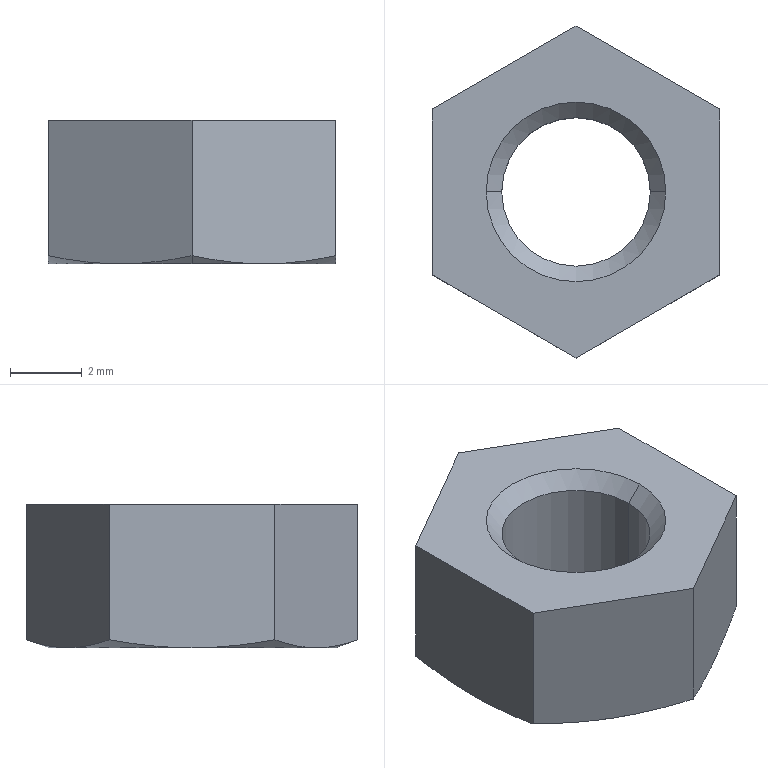Part | SolidWorks | features BaseBody 1 | 1 solid | 21 faces | box 8 x 9.238 x 4 mm | volume 165.049 mm3 | cone 11 | plane 8 | cylinder 2 | commonest cylinder face diameters 4.134 x2
STEP:
#1=CARTESIAN_POINT('',(-2.067,0.,0.433));
#2=VERTEX_POINT('',#1);
#3=CARTESIAN_POINT('',(2.067,0.,0.433));
#4=VERTEX_POINT('',#3);
#5=CARTESIAN_POINT('',(0.,0.,0.433));
#6=DIRECTION('',(0.,0.,1.));
#7=DIRECTION('',(1.,0.,0.));
#8=AXIS2_PLACEMENT_3D('',#5,#6,#7);
#9=CIRCLE('',#8,2.067);
#10=EDGE_CURVE('',#2,#4,#9,.T.);
#11=ORIENTED_EDGE('',*,*,#10,.F.);
#12=CARTESIAN_POINT('',(-2.067,0.,3.567));
#13=VERTEX_POINT('',#12);
#14=CARTESIAN_POINT('',(-2.067,0.,0.));
#15=DIRECTION('',(0.,0.,1.));
#16=VECTOR('',#15,1000.);
#17=LINE('',#14,#16);
#18=EDGE_CURVE('',#2,#13,#17,.T.);
#19=ORIENTED_EDGE('',*,*,#18,.T.);
#20=CARTESIAN_POINT('',(2.067,0.,3.567));
#21=VERTEX_POINT('',#20);
#22=CARTESIAN_POINT('',(0.,0.,3.567));
#23=DIRECTION('',(0.,0.,-1.));
#24=DIRECTION('',(1.,0.,0.));
#25=AXIS2_PLACEMENT_3D('',#22,#23,#24);
#26=CIRCLE('',#25,2.067);
#27=EDGE_CURVE('',#21,#13,#26,.T.);
#28=ORIENTED_EDGE('',*,*,#27,.F.);
#29=CARTESIAN_POINT('',(2.067,0.,0.));
#30=DIRECTION('',(0.,0.,1.));
#31=VECTOR('',#30,1000.);
#32=LINE('',#29,#31);
#33=EDGE_CURVE('',#4,#21,#32,.T.);
#34=ORIENTED_EDGE('',*,*,#33,.F.);
#35=EDGE_LOOP('',(#11,#19,#28,#34));
#36=FACE_OUTER_BOUND('',#35,.T.);
#37=CARTESIAN_POINT('',(0.,0.,0.));
#38=DIRECTION('',(0.,0.,1.));
#39=DIRECTION('',(1.,0.,0.));
#40=AXIS2_PLACEMENT_3D('',#37,#38,#39);
#41=CYLINDRICAL_SURFACE('',#40,2.067);
#42=ADVANCED_FACE('',(#36),#41,.F.);
#43=ORIENTED_EDGE('',*,*,#27,.T.);
#44=CARTESIAN_POINT('',(-2.5,0.,4.));
#45=VERTEX_POINT('',#44);
#46=CARTESIAN_POINT('',(-2.5,0.,4.));
#47=DIRECTION('',(-0.7071,0.,0.7071));
#48=VECTOR('',#47,1000.);
#49=LINE('',#46,#48);
#50=EDGE_CURVE('',#13,#45,#49,.T.);
#51=ORIENTED_EDGE('',*,*,#50,.T.);
#52=CARTESIAN_POINT('',(2.5,0.,4.));
#53=VERTEX_POINT('',#52);
#54=CARTESIAN_POINT('',(0.,0.,4.));
#55=DIRECTION('',(0.,0.,-1.));
#56=DIRECTION('',(1.,0.,0.));
#57=AXIS2_PLACEMENT_3D('',#54,#55,#56);
#58=CIRCLE('',#57,2.5);
#59=EDGE_CURVE('',#53,#45,#58,.T.);
#60=ORIENTED_EDGE('',*,*,#59,.F.);
#61=CARTESIAN_POINT('',(2.5,0.,4.));
#62=DIRECTION('',(0.7071,0.,0.7071));
#63=VECTOR('',#62,1000.);
#64=LINE('',#61,#63);
#65=EDGE_CURVE('',#21,#53,#64,.T.);
#66=ORIENTED_EDGE('',*,*,#65,.F.);
#67=EDGE_LOOP('',(#43,#51,#60,#66));
#68=FACE_OUTER_BOUND('',#67,.T.);
#69=CARTESIAN_POINT('',(0.,0.,4.));
#70=DIRECTION('',(0.,0.,1.));
#71=DIRECTION('',(1.,0.,0.));
#72=AXIS2_PLACEMENT_3D('',#69,#70,#71);
#73=CONICAL_SURFACE('',#72,2.5,0.7854);
#74=ADVANCED_FACE('',(#68),#73,.F.);
#75=ORIENTED_EDGE('',*,*,#10,.T.);
#76=CARTESIAN_POINT('',(2.5,0.,0.));
#77=VERTEX_POINT('',#76);
#78=CARTESIAN_POINT('',(2.5,0.,0.));
#79=DIRECTION('',(0.7071,0.,-0.7071));
#80=VECTOR('',#79,1000.);
#81=LINE('',#78,#80);
#82=EDGE_CURVE('',#4,#77,#81,.T.);
#83=ORIENTED_EDGE('',*,*,#82,.T.);
#84=CARTESIAN_POINT('',(-2.5,0.,0.));
#85=VERTEX_POINT('',#84);
#86=CARTESIAN_POINT('',(0.,0.,0.));
#87=DIRECTION('',(0.,0.,1.));
#88=DIRECTION('',(-1.,0.,0.));
#89=AXIS2_PLACEMENT_3D('',#86,#87,#88);
#90=CIRCLE('',#89,2.5);
#91=EDGE_CURVE('',#85,#77,#90,.T.);
#92=ORIENTED_EDGE('',*,*,#91,.F.);
#93=CARTESIAN_POINT('',(-2.5,0.,0.));
#94=DIRECTION('',(-0.7071,0.,-0.7071));
#95=VECTOR('',#94,1000.);
#96=LINE('',#93,#95);
#97=EDGE_CURVE('',#2,#85,#96,.T.);
#98=ORIENTED_EDGE('',*,*,#97,.F.);
#99=EDGE_LOOP('',(#75,#83,#92,#98));
#100=FACE_OUTER_BOUND('',#99,.T.);
#101=CARTESIAN_POINT('',(0.,0.,0.));
#102=DIRECTION('',(0.,0.,-1.));
#103=DIRECTION('',(-1.,0.,0.));
#104=AXIS2_PLACEMENT_3D('',#101,#102,#103);
#105=CONICAL_SURFACE('',#104,2.5,0.7854);
#106=ADVANCED_FACE('',(#100),#105,.F.);
#107=CARTESIAN_POINT('',(-2.,-3.464,0.));
#108=VERTEX_POINT('',#107);
#109=CARTESIAN_POINT('',(0.,-4.,0.));
#110=VERTEX_POINT('',#109);
#111=CARTESIAN_POINT('',(0.,0.,0.));
#112=DIRECTION('',(0.,0.,1.));
#113=DIRECTION('',(0.,-1.,0.));
#114=AXIS2_PLACEMENT_3D('',#111,#112,#113);
#115=CIRCLE('',#114,4.);
#116=EDGE_CURVE('',#108,#110,#115,.T.);
#117=ORIENTED_EDGE('',*,*,#116,.T.);
#118=CARTESIAN_POINT('',(0.,-4.619,0.2252));
#119=VERTEX_POINT('',#118);
#120=CARTESIAN_POINT('',(0.,-4.623,0.2266));
#121=DIRECTION('',(0.,-0.9397,0.342));
#122=VECTOR('',#121,1000.);
#123=LINE('',#120,#122);
#124=EDGE_CURVE('',#110,#119,#123,.T.);
#125=ORIENTED_EDGE('',*,*,#124,.T.);
#126=CARTESIAN_POINT('',(0.,-4.619,0.2252));
#127=CARTESIAN_POINT('',(-0.6613,-4.237,0.08627));
#128=CARTESIAN_POINT('',(-1.327,-3.853,0.));
#129=CARTESIAN_POINT('',(-2.,-3.464,0.));
#130=B_SPLINE_CURVE_WITH_KNOTS('',3,(#126,#127,#128,#129),.UNSPECIFIED.,.F.,.F.,(4,4),(0.,0.00232),.UNSPECIFIED.);
#131=EDGE_CURVE('',#119,#108,#130,.T.);
#132=ORIENTED_EDGE('',*,*,#131,.T.);
#133=EDGE_LOOP('',(#117,#125,#132));
#134=FACE_OUTER_BOUND('',#133,.T.);
#135=CARTESIAN_POINT('',(0.,0.,0.2266));
#136=DIRECTION('',(0.,0.,1.));
#137=DIRECTION('',(0.,-1.,0.));
#138=AXIS2_PLACEMENT_3D('',#135,#136,#137);
#139=CONICAL_SURFACE('',#138,4.623,1.222);
#140=ADVANCED_FACE('',(#134),#139,.T.);
#141=ORIENTED_EDGE('',*,*,#18,.F.);
#142=CARTESIAN_POINT('',(0.,0.,0.433));
#143=DIRECTION('',(0.,0.,1.));
#144=DIRECTION('',(1.,0.,0.));
#145=AXIS2_PLACEMENT_3D('',#142,#143,#144);
#146=CIRCLE('',#145,2.067);
#147=EDGE_CURVE('',#4,#2,#146,.T.);
#148=ORIENTED_EDGE('',*,*,#147,.F.);
#149=ORIENTED_EDGE('',*,*,#33,.T.);
#150=CARTESIAN_POINT('',(0.,0.,3.567));
#151=DIRECTION('',(0.,0.,-1.));
#152=DIRECTION('',(1.,0.,0.));
#153=AXIS2_PLACEMENT_3D('',#150,#151,#152);
#154=CIRCLE('',#153,2.067);
#155=EDGE_CURVE('',#13,#21,#154,.T.);
#156=ORIENTED_EDGE('',*,*,#155,.F.);
#157=EDGE_LOOP('',(#141,#148,#149,#156));
#158=FACE_OUTER_BOUND('',#157,.T.);
#159=CARTESIAN_POINT('',(0.,0.,0.));
#160=DIRECTION('',(0.,0.,1.));
#161=DIRECTION('',(1.,0.,0.));
#162=AXIS2_PLACEMENT_3D('',#159,#160,#161);
#163=CYLINDRICAL_SURFACE('',#162,2.067);
#164=ADVANCED_FACE('',(#158),#163,.F.);
#165=ORIENTED_EDGE('',*,*,#50,.F.);
#166=ORIENTED_EDGE('',*,*,#155,.T.);
#167=ORIENTED_EDGE('',*,*,#65,.T.);
#168=CARTESIAN_POINT('',(0.,0.,4.));
#169=DIRECTION('',(0.,0.,-1.));
#170=DIRECTION('',(1.,0.,0.));
#171=AXIS2_PLACEMENT_3D('',#168,#169,#170);
#172=CIRCLE('',#171,2.5);
#173=EDGE_CURVE('',#45,#53,#172,.T.);
#174=ORIENTED_EDGE('',*,*,#173,.F.);
#175=EDGE_LOOP('',(#165,#166,#167,#174));
#176=FACE_OUTER_BOUND('',#175,.T.);
#177=CARTESIAN_POINT('',(0.,0.,4.));
#178=DIRECTION('',(0.,0.,1.));
#179=DIRECTION('',(1.,0.,0.));
#180=AXIS2_PLACEMENT_3D('',#177,#178,#179);
#181=CONICAL_SURFACE('',#180,2.5,0.7854);
#182=ADVANCED_FACE('',(#176),#181,.F.);
#183=ORIENTED_EDGE('',*,*,#82,.F.);
#184=ORIENTED_EDGE('',*,*,#147,.T.);
#185=ORIENTED_EDGE('',*,*,#97,.T.);
#186=CARTESIAN_POINT('',(0.,0.,0.));
#187=DIRECTION('',(0.,0.,1.));
#188=DIRECTION('',(-1.,0.,0.));
#189=AXIS2_PLACEMENT_3D('',#186,#187,#188);
#190=CIRCLE('',#189,2.5);
#191=EDGE_CURVE('',#77,#85,#190,.T.);
#192=ORIENTED_EDGE('',*,*,#191,.F.);
#193=EDGE_LOOP('',(#183,#184,#185,#192));
#194=FACE_OUTER_BOUND('',#193,.T.);
#195=CARTESIAN_POINT('',(0.,0.,0.));
#196=DIRECTION('',(0.,0.,-1.));
#197=DIRECTION('',(-1.,0.,0.));
#198=AXIS2_PLACEMENT_3D('',#195,#196,#197);
#199=CONICAL_SURFACE('',#198,2.5,0.7854);
#200=ADVANCED_FACE('',(#194),#199,.F.);
#201=ORIENTED_EDGE('',*,*,#59,.T.);
#202=ORIENTED_EDGE('',*,*,#173,.T.);
#203=EDGE_LOOP('',(#201,#202));
#204=FACE_BOUND('',#203,.T.);
#205=CARTESIAN_POINT('',(4.,-2.309,4.));
#206=VERTEX_POINT('',#205);
#207=CARTESIAN_POINT('',(4.,2.309,4.));
#208=VERTEX_POINT('',#207);
#209=CARTESIAN_POINT('',(4.,0.,4.));
#210=DIRECTION('',(0.,1.,0.));
#211=VECTOR('',#210,1000.);
#212=LINE('',#209,#211);
#213=EDGE_CURVE('',#206,#208,#212,.T.);
#214=ORIENTED_EDGE('',*,*,#213,.T.);
#215=CARTESIAN_POINT('',(0.,4.619,4.));
#216=VERTEX_POINT('',#215);
#217=CARTESIAN_POINT('',(4.,2.309,4.));
#218=DIRECTION('',(-0.866,0.5,0.));
#219=VECTOR('',#218,1000.);
#220=LINE('',#217,#219);
#221=EDGE_CURVE('',#208,#216,#220,.T.);
#222=ORIENTED_EDGE('',*,*,#221,.T.);
#223=CARTESIAN_POINT('',(-4.,2.309,4.));
#224=VERTEX_POINT('',#223);
#225=CARTESIAN_POINT('',(0.,4.619,4.));
#226=DIRECTION('',(-0.866,-0.5,0.));
#227=VECTOR('',#226,1000.);
#228=LINE('',#225,#227);
#229=EDGE_CURVE('',#216,#224,#228,.T.);
#230=ORIENTED_EDGE('',*,*,#229,.T.);
#231=CARTESIAN_POINT('',(-4.,-2.309,4.));
#232=VERTEX_POINT('',#231);
#233=CARTESIAN_POINT('',(-4.,0.,4.));
#234=DIRECTION('',(0.,-1.,0.));
#235=VECTOR('',#234,1000.);
#236=LINE('',#233,#235);
#237=EDGE_CURVE('',#224,#232,#236,.T.);
#238=ORIENTED_EDGE('',*,*,#237,.T.);
#239=CARTESIAN_POINT('',(0.,-4.619,4.));
#240=VERTEX_POINT('',#239);
#241=CARTESIAN_POINT('',(-4.,-2.309,4.));
#242=DIRECTION('',(0.866,-0.5,0.));
#243=VECTOR('',#242,1000.);
#244=LINE('',#241,#243);
#245=EDGE_CURVE('',#232,#240,#244,.T.);
#246=ORIENTED_EDGE('',*,*,#245,.T.);
#247=CARTESIAN_POINT('',(0.,-4.619,4.));
#248=DIRECTION('',(0.866,0.5,0.));
#249=VECTOR('',#248,1000.);
#250=LINE('',#247,#249);
#251=EDGE_CURVE('',#240,#206,#250,.T.);
#252=ORIENTED_EDGE('',*,*,#251,.T.);
#253=EDGE_LOOP('',(#214,#222,#230,#238,#246,#252));
#254=FACE_OUTER_BOUND('',#253,.T.);
#255=CARTESIAN_POINT('',(0.,0.,4.));
#256=DIRECTION('',(0.,0.,1.));
#257=DIRECTION('',(1.,0.,0.));
#258=AXIS2_PLACEMENT_3D('',#255,#256,#257);
#259=PLANE('',#258);
#260=ADVANCED_FACE('',(#204,#254),#259,.T.);
#261=ORIENTED_EDGE('',*,*,#91,.T.);
#262=ORIENTED_EDGE('',*,*,#191,.T.);
#263=EDGE_LOOP('',(#261,#262));
#264=FACE_BOUND('',#263,.T.);
#265=ORIENTED_EDGE('',*,*,#116,.F.);
#266=CARTESIAN_POINT('',(-4.,0.,0.));
#267=VERTEX_POINT('',#266);
#268=CARTESIAN_POINT('',(0.,0.,0.));
#269=DIRECTION('',(0.,0.,1.));
#270=DIRECTION('',(0.,-1.,0.));
#271=AXIS2_PLACEMENT_3D('',#268,#269,#270);
#272=CIRCLE('',#271,4.);
#273=EDGE_CURVE('',#267,#108,#272,.T.);
#274=ORIENTED_EDGE('',*,*,#273,.F.);
#275=CARTESIAN_POINT('',(-2.,3.464,0.));
#276=VERTEX_POINT('',#275);
#277=CARTESIAN_POINT('',(0.,0.,0.));
#278=DIRECTION('',(0.,0.,1.));
#279=DIRECTION('',(0.,-1.,0.));
#280=AXIS2_PLACEMENT_3D('',#277,#278,#279);
#281=CIRCLE('',#280,4.);
#282=EDGE_CURVE('',#276,#267,#281,.T.);
#283=ORIENTED_EDGE('',*,*,#282,.F.);
#284=CARTESIAN_POINT('',(2.,3.464,0.));
#285=VERTEX_POINT('',#284);
#286=CARTESIAN_POINT('',(0.,0.,0.));
#287=DIRECTION('',(0.,0.,1.));
#288=DIRECTION('',(0.,-1.,0.));
#289=AXIS2_PLACEMENT_3D('',#286,#287,#288);
#290=CIRCLE('',#289,4.);
#291=EDGE_CURVE('',#285,#276,#290,.T.);
#292=ORIENTED_EDGE('',*,*,#291,.F.);
#293=CARTESIAN_POINT('',(4.,0.,0.));
#294=VERTEX_POINT('',#293);
#295=CARTESIAN_POINT('',(0.,0.,0.));
#296=DIRECTION('',(0.,0.,1.));
#297=DIRECTION('',(0.,-1.,0.));
#298=AXIS2_PLACEMENT_3D('',#295,#296,#297);
#299=CIRCLE('',#298,4.);
#300=EDGE_CURVE('',#294,#285,#299,.T.);
#301=ORIENTED_EDGE('',*,*,#300,.F.);
#302=CARTESIAN_POINT('',(2.,-3.464,0.));
#303=VERTEX_POINT('',#302);
#304=CARTESIAN_POINT('',(0.,0.,0.));
#305=DIRECTION('',(0.,0.,1.));
#306=DIRECTION('',(0.,-1.,0.));
#307=AXIS2_PLACEMENT_3D('',#304,#305,#306);
#308=CIRCLE('',#307,4.);
#309=EDGE_CURVE('',#303,#294,#308,.T.);
#310=ORIENTED_EDGE('',*,*,#309,.F.);
#311=CARTESIAN_POINT('',(0.,0.,0.));
#312=DIRECTION('',(0.,0.,1.));
#313=DIRECTION('',(0.,-1.,0.));
#314=AXIS2_PLACEMENT_3D('',#311,#312,#313);
#315=CIRCLE('',#314,4.);
#316=EDGE_CURVE('',#110,#303,#315,.T.);
#317=ORIENTED_EDGE('',*,*,#316,.F.);
#318=EDGE_LOOP('',(#265,#274,#283,#292,#301,#310,#317));
#319=FACE_OUTER_BOUND('',#318,.T.);
#320=CARTESIAN_POINT('',(0.,0.,0.));
#321=DIRECTION('',(0.,0.,1.));
#322=DIRECTION('',(1.,0.,0.));
#323=AXIS2_PLACEMENT_3D('',#320,#321,#322);
#324=PLANE('',#323);
#325=ADVANCED_FACE('',(#264,#319),#324,.F.);
#326=CARTESIAN_POINT('',(4.,2.309,0.2252));
#327=VERTEX_POINT('',#326);
#328=CARTESIAN_POINT('',(2.,3.464,0.));
#329=CARTESIAN_POINT('',(2.673,3.076,0.));
#330=CARTESIAN_POINT('',(3.339,2.691,0.08627));
#331=CARTESIAN_POINT('',(4.,2.309,0.2252));
#332=B_SPLINE_CURVE_WITH_KNOTS('',3,(#328,#329,#330,#331),.UNSPECIFIED.,.F.,.F.,(4,4),(0.,0.00232),.UNSPECIFIED.);
#333=EDGE_CURVE('',#285,#327,#332,.T.);
#334=ORIENTED_EDGE('',*,*,#333,.F.);
#335=CARTESIAN_POINT('',(0.,4.619,0.2252));
#336=VERTEX_POINT('',#335);
#337=CARTESIAN_POINT('',(0.,4.619,0.2252));
#338=CARTESIAN_POINT('',(0.6613,4.237,0.08627));
#339=CARTESIAN_POINT('',(1.327,3.853,0.));
#340=CARTESIAN_POINT('',(2.,3.464,0.));
#341=B_SPLINE_CURVE_WITH_KNOTS('',3,(#337,#338,#339,#340),.UNSPECIFIED.,.F.,.F.,(4,4),(0.,0.00232),.UNSPECIFIED.);
#342=EDGE_CURVE('',#336,#285,#341,.T.);
#343=ORIENTED_EDGE('',*,*,#342,.F.);
#344=CARTESIAN_POINT('',(0.,4.619,4.));
#345=DIRECTION('',(0.,0.,-1.));
#346=VECTOR('',#345,1000.);
#347=LINE('',#344,#346);
#348=EDGE_CURVE('',#216,#336,#347,.T.);
#349=ORIENTED_EDGE('',*,*,#348,.F.);
#350=ORIENTED_EDGE('',*,*,#221,.F.);
#351=CARTESIAN_POINT('',(4.,2.309,4.));
#352=DIRECTION('',(0.,0.,1.));
#353=VECTOR('',#352,1000.);
#354=LINE('',#351,#353);
#355=EDGE_CURVE('',#327,#208,#354,.T.);
#356=ORIENTED_EDGE('',*,*,#355,.F.);
#357=EDGE_LOOP('',(#334,#343,#349,#350,#356));
#358=FACE_OUTER_BOUND('',#357,.T.);
#359=CARTESIAN_POINT('',(4.,2.309,4.));
#360=DIRECTION('',(-0.5,-0.866,0.));
#361=DIRECTION('',(0.866,-0.5,0.));
#362=AXIS2_PLACEMENT_3D('',#359,#360,#361);
#363=PLANE('',#362);
#364=ADVANCED_FACE('',(#358),#363,.F.);
#365=CARTESIAN_POINT('',(4.,-2.309,0.2252));
#366=VERTEX_POINT('',#365);
#367=CARTESIAN_POINT('',(4.,0.,0.));
#368=CARTESIAN_POINT('',(4.,-0.7771,0.));
#369=CARTESIAN_POINT('',(4.,-1.546,0.08627));
#370=CARTESIAN_POINT('',(4.,-2.309,0.2252));
#371=B_SPLINE_CURVE_WITH_KNOTS('',3,(#367,#368,#369,#370),.UNSPECIFIED.,.F.,.F.,(4,4),(0.,0.00232),.UNSPECIFIED.);
#372=EDGE_CURVE('',#294,#366,#371,.T.);
#373=ORIENTED_EDGE('',*,*,#372,.F.);
#374=CARTESIAN_POINT('',(4.,2.309,0.2252));
#375=CARTESIAN_POINT('',(4.,1.546,0.08627));
#376=CARTESIAN_POINT('',(4.,0.7771,0.));
#377=CARTESIAN_POINT('',(4.,0.,0.));
#378=B_SPLINE_CURVE_WITH_KNOTS('',3,(#374,#375,#376,#377),.UNSPECIFIED.,.F.,.F.,(4,4),(0.,0.00232),.UNSPECIFIED.);
#379=EDGE_CURVE('',#327,#294,#378,.T.);
#380=ORIENTED_EDGE('',*,*,#379,.F.);
#381=ORIENTED_EDGE('',*,*,#355,.T.);
#382=ORIENTED_EDGE('',*,*,#213,.F.);
#383=CARTESIAN_POINT('',(4.,-2.309,4.));
#384=DIRECTION('',(0.,0.,1.));
#385=VECTOR('',#384,1000.);
#386=LINE('',#383,#385);
#387=EDGE_CURVE('',#366,#206,#386,.T.);
#388=ORIENTED_EDGE('',*,*,#387,.F.);
#389=EDGE_LOOP('',(#373,#380,#381,#382,#388));
#390=FACE_OUTER_BOUND('',#389,.T.);
#391=CARTESIAN_POINT('',(4.,-2.309,4.));
#392=DIRECTION('',(-1.,0.,0.));
#393=DIRECTION('',(0.,0.,1.));
#394=AXIS2_PLACEMENT_3D('',#391,#392,#393);
#395=PLANE('',#394);
#396=ADVANCED_FACE('',(#390),#395,.F.);
#397=CARTESIAN_POINT('',(2.,-3.464,0.));
#398=CARTESIAN_POINT('',(1.327,-3.853,0.));
#399=CARTESIAN_POINT('',(0.6613,-4.237,0.08627));
#400=CARTESIAN_POINT('',(0.,-4.619,0.2252));
#401=B_SPLINE_CURVE_WITH_KNOTS('',3,(#397,#398,#399,#400),.UNSPECIFIED.,.F.,.F.,(4,4),(0.,0.00232),.UNSPECIFIED.);
#402=EDGE_CURVE('',#303,#119,#401,.T.);
#403=ORIENTED_EDGE('',*,*,#402,.F.);
#404=CARTESIAN_POINT('',(4.,-2.309,0.2252));
#405=CARTESIAN_POINT('',(3.339,-2.691,0.08627));
#406=CARTESIAN_POINT('',(2.673,-3.076,0.));
#407=CARTESIAN_POINT('',(2.,-3.464,0.));
#408=B_SPLINE_CURVE_WITH_KNOTS('',3,(#404,#405,#406,#407),.UNSPECIFIED.,.F.,.F.,(4,4),(0.,0.00232),.UNSPECIFIED.);
#409=EDGE_CURVE('',#366,#303,#408,.T.);
#410=ORIENTED_EDGE('',*,*,#409,.F.);
#411=ORIENTED_EDGE('',*,*,#387,.T.);
#412=ORIENTED_EDGE('',*,*,#251,.F.);
#413=CARTESIAN_POINT('',(0.,-4.619,4.));
#414=DIRECTION('',(0.,0.,1.));
#415=VECTOR('',#414,1000.);
#416=LINE('',#413,#415);
#417=EDGE_CURVE('',#119,#240,#416,.T.);
#418=ORIENTED_EDGE('',*,*,#417,.F.);
#419=EDGE_LOOP('',(#403,#410,#411,#412,#418));
#420=FACE_OUTER_BOUND('',#419,.T.);
#421=CARTESIAN_POINT('',(0.,-4.619,4.));
#422=DIRECTION('',(-0.5,0.866,0.));
#423=DIRECTION('',(-0.866,-0.5,0.));
#424=AXIS2_PLACEMENT_3D('',#421,#422,#423);
#425=PLANE('',#424);
#426=ADVANCED_FACE('',(#420),#425,.F.);
#427=CARTESIAN_POINT('',(-4.,-2.309,0.2252));
#428=VERTEX_POINT('',#427);
#429=CARTESIAN_POINT('',(-2.,-3.464,0.));
#430=CARTESIAN_POINT('',(-2.673,-3.076,0.));
#431=CARTESIAN_POINT('',(-3.339,-2.691,0.08627));
#432=CARTESIAN_POINT('',(-4.,-2.309,0.2252));
#433=B_SPLINE_CURVE_WITH_KNOTS('',3,(#429,#430,#431,#432),.UNSPECIFIED.,.F.,.F.,(4,4),(0.,0.00232),.UNSPECIFIED.);
#434=EDGE_CURVE('',#108,#428,#433,.T.);
#435=ORIENTED_EDGE('',*,*,#434,.F.);
#436=ORIENTED_EDGE('',*,*,#131,.F.);
#437=ORIENTED_EDGE('',*,*,#417,.T.);
#438=ORIENTED_EDGE('',*,*,#245,.F.);
#439=CARTESIAN_POINT('',(-4.,-2.309,4.));
#440=DIRECTION('',(0.,0.,1.));
#441=VECTOR('',#440,1000.);
#442=LINE('',#439,#441);
#443=EDGE_CURVE('',#428,#232,#442,.T.);
#444=ORIENTED_EDGE('',*,*,#443,.F.);
#445=EDGE_LOOP('',(#435,#436,#437,#438,#444));
#446=FACE_OUTER_BOUND('',#445,.T.);
#447=CARTESIAN_POINT('',(-4.,-2.309,4.));
#448=DIRECTION('',(0.5,0.866,0.));
#449=DIRECTION('',(-0.866,0.5,0.));
#450=AXIS2_PLACEMENT_3D('',#447,#448,#449);
#451=PLANE('',#450);
#452=ADVANCED_FACE('',(#446),#451,.F.);
#453=CARTESIAN_POINT('',(-4.,2.309,0.2252));
#454=VERTEX_POINT('',#453);
#455=CARTESIAN_POINT('',(-4.,0.,0.));
#456=CARTESIAN_POINT('',(-4.,0.7771,0.));
#457=CARTESIAN_POINT('',(-4.,1.546,0.08627));
#458=CARTESIAN_POINT('',(-4.,2.309,0.2252));
#459=B_SPLINE_CURVE_WITH_KNOTS('',3,(#455,#456,#457,#458),.UNSPECIFIED.,.F.,.F.,(4,4),(0.,0.00232),.UNSPECIFIED.);
#460=EDGE_CURVE('',#267,#454,#459,.T.);
#461=ORIENTED_EDGE('',*,*,#460,.F.);
#462=CARTESIAN_POINT('',(-4.,-2.309,0.2252));
#463=CARTESIAN_POINT('',(-4.,-1.546,0.08627));
#464=CARTESIAN_POINT('',(-4.,-0.7771,0.));
#465=CARTESIAN_POINT('',(-4.,0.,0.));
#466=B_SPLINE_CURVE_WITH_KNOTS('',3,(#462,#463,#464,#465),.UNSPECIFIED.,.F.,.F.,(4,4),(0.,0.00232),.UNSPECIFIED.);
#467=EDGE_CURVE('',#428,#267,#466,.T.);
#468=ORIENTED_EDGE('',*,*,#467,.F.);
#469=ORIENTED_EDGE('',*,*,#443,.T.);
#470=ORIENTED_EDGE('',*,*,#237,.F.);
#471=CARTESIAN_POINT('',(-4.,2.309,4.));
#472=DIRECTION('',(0.,0.,1.));
#473=VECTOR('',#472,1000.);
#474=LINE('',#471,#473);
#475=EDGE_CURVE('',#454,#224,#474,.T.);
#476=ORIENTED_EDGE('',*,*,#475,.F.);
#477=EDGE_LOOP('',(#461,#468,#469,#470,#476));
#478=FACE_OUTER_BOUND('',#477,.T.);
#479=CARTESIAN_POINT('',(-4.,2.309,4.));
#480=DIRECTION('',(1.,0.,0.));
#481=DIRECTION('',(0.,0.,-1.));
#482=AXIS2_PLACEMENT_3D('',#479,#480,#481);
#483=PLANE('',#482);
#484=ADVANCED_FACE('',(#478),#483,.F.);
#485=CARTESIAN_POINT('',(-2.,3.464,0.));
#486=CARTESIAN_POINT('',(-1.327,3.853,0.));
#487=CARTESIAN_POINT('',(-0.6613,4.237,0.08627));
#488=CARTESIAN_POINT('',(0.,4.619,0.2252));
#489=B_SPLINE_CURVE_WITH_KNOTS('',3,(#485,#486,#487,#488),.UNSPECIFIED.,.F.,.F.,(4,4),(0.,0.00232),.UNSPECIFIED.);
#490=EDGE_CURVE('',#276,#336,#489,.T.);
#491=ORIENTED_EDGE('',*,*,#490,.F.);
#492=CARTESIAN_POINT('',(-4.,2.309,0.2252));
#493=CARTESIAN_POINT('',(-3.339,2.691,0.08627));
#494=CARTESIAN_POINT('',(-2.673,3.076,0.));
#495=CARTESIAN_POINT('',(-2.,3.464,0.));
#496=B_SPLINE_CURVE_WITH_KNOTS('',3,(#492,#493,#494,#495),.UNSPECIFIED.,.F.,.F.,(4,4),(0.,0.00232),.UNSPECIFIED.);
#497=EDGE_CURVE('',#454,#276,#496,.T.);
#498=ORIENTED_EDGE('',*,*,#497,.F.);
#499=ORIENTED_EDGE('',*,*,#475,.T.);
#500=ORIENTED_EDGE('',*,*,#229,.F.);
#501=ORIENTED_EDGE('',*,*,#348,.T.);
#502=EDGE_LOOP('',(#491,#498,#499,#500,#501));
#503=FACE_OUTER_BOUND('',#502,.T.);
#504=CARTESIAN_POINT('',(0.,4.619,4.));
#505=DIRECTION('',(0.5,-0.866,0.));
#506=DIRECTION('',(0.866,0.5,0.));
#507=AXIS2_PLACEMENT_3D('',#504,#505,#506);
#508=PLANE('',#507);
#509=ADVANCED_FACE('',(#503),#508,.F.);
#510=ORIENTED_EDGE('',*,*,#372,.T.);
#511=ORIENTED_EDGE('',*,*,#409,.T.);
#512=ORIENTED_EDGE('',*,*,#309,.T.);
#513=EDGE_LOOP('',(#510,#511,#512));
#514=FACE_OUTER_BOUND('',#513,.T.);
#515=CARTESIAN_POINT('',(0.,0.,0.2266));
#516=DIRECTION('',(0.,0.,1.));
#517=DIRECTION('',(0.,-1.,0.));
#518=AXIS2_PLACEMENT_3D('',#515,#516,#517);
#519=CONICAL_SURFACE('',#518,4.623,1.222);
#520=ADVANCED_FACE('',(#514),#519,.T.);
#521=ORIENTED_EDGE('',*,*,#124,.F.);
#522=ORIENTED_EDGE('',*,*,#316,.T.);
#523=ORIENTED_EDGE('',*,*,#402,.T.);
#524=EDGE_LOOP('',(#521,#522,#523));
#525=FACE_OUTER_BOUND('',#524,.T.);
#526=CARTESIAN_POINT('',(0.,0.,0.2266));
#527=DIRECTION('',(0.,0.,1.));
#528=DIRECTION('',(0.,-1.,0.));
#529=AXIS2_PLACEMENT_3D('',#526,#527,#528);
#530=CONICAL_SURFACE('',#529,4.623,1.222);
#531=ADVANCED_FACE('',(#525),#530,.T.);
#532=ORIENTED_EDGE('',*,*,#434,.T.);
#533=ORIENTED_EDGE('',*,*,#467,.T.);
#534=ORIENTED_EDGE('',*,*,#273,.T.);
#535=EDGE_LOOP('',(#532,#533,#534));
#536=FACE_OUTER_BOUND('',#535,.T.);
#537=CARTESIAN_POINT('',(0.,0.,0.2266));
#538=DIRECTION('',(0.,0.,1.));
#539=DIRECTION('',(0.,-1.,0.));
#540=AXIS2_PLACEMENT_3D('',#537,#538,#539);
#541=CONICAL_SURFACE('',#540,4.623,1.222);
#542=ADVANCED_FACE('',(#536),#541,.T.);
#543=ORIENTED_EDGE('',*,*,#460,.T.);
#544=ORIENTED_EDGE('',*,*,#497,.T.);
#545=ORIENTED_EDGE('',*,*,#282,.T.);
#546=EDGE_LOOP('',(#543,#544,#545));
#547=FACE_OUTER_BOUND('',#546,.T.);
#548=CARTESIAN_POINT('',(0.,0.,0.2266));
#549=DIRECTION('',(0.,0.,1.));
#550=DIRECTION('',(0.,-1.,0.));
#551=AXIS2_PLACEMENT_3D('',#548,#549,#550);
#552=CONICAL_SURFACE('',#551,4.623,1.222);
#553=ADVANCED_FACE('',(#547),#552,.T.);
#554=ORIENTED_EDGE('',*,*,#342,.T.);
#555=ORIENTED_EDGE('',*,*,#291,.T.);
#556=ORIENTED_EDGE('',*,*,#490,.T.);
#557=EDGE_LOOP('',(#554,#555,#556));
#558=FACE_OUTER_BOUND('',#557,.T.);
#559=CARTESIAN_POINT('',(0.,0.,0.2266));
#560=DIRECTION('',(0.,0.,1.));
#561=DIRECTION('',(0.,-1.,0.));
#562=AXIS2_PLACEMENT_3D('',#559,#560,#561);
#563=CONICAL_SURFACE('',#562,4.623,1.222);
#564=ADVANCED_FACE('',(#558),#563,.T.);
#565=ORIENTED_EDGE('',*,*,#333,.T.);
#566=ORIENTED_EDGE('',*,*,#379,.T.);
#567=ORIENTED_EDGE('',*,*,#300,.T.);
#568=EDGE_LOOP('',(#565,#566,#567));
#569=FACE_OUTER_BOUND('',#568,.T.);
#570=CARTESIAN_POINT('',(0.,0.,0.2266));
#571=DIRECTION('',(0.,0.,1.));
#572=DIRECTION('',(0.,-1.,0.));
#573=AXIS2_PLACEMENT_3D('',#570,#571,#572);
#574=CONICAL_SURFACE('',#573,4.623,1.222);
#575=ADVANCED_FACE('',(#569),#574,.T.);
#576=CLOSED_SHELL('',(#42,#74,#106,#140,#164,#182,#200,#260,#325,#364,#396,#426,#452,#484,#509,#520,#531,#542,#553,#564,#575));
#577=MANIFOLD_SOLID_BREP('',#576);
#578=CARTESIAN_POINT('',(0.,0.,0.));
#579=DIRECTION('',(0.,0.,1.));
#580=DIRECTION('',(1.,0.,0.));
#581=AXIS2_PLACEMENT_3D('',#578,#579,#580);
#582=(LENGTH_UNIT()NAMED_UNIT(*)SI_UNIT(.MILLI.,.METRE.));
#583=UNCERTAINTY_MEASURE_WITH_UNIT(LENGTH_MEASURE(0.00001),#582,'','');
#584=(NAMED_UNIT(*)PLANE_ANGLE_UNIT()SI_UNIT($,.RADIAN.));
#585=(NAMED_UNIT(*)SI_UNIT($,.STERADIAN.)SOLID_ANGLE_UNIT());
#586=(GEOMETRIC_REPRESENTATION_CONTEXT(3)GLOBAL_UNCERTAINTY_ASSIGNED_CONTEXT((#583))GLOBAL_UNIT_ASSIGNED_CONTEXT((#582,#584,#585))REPRESENTATION_CONTEXT('',''));
#587=ADVANCED_BREP_SHAPE_REPRESENTATION('',(#577,#581),#586);